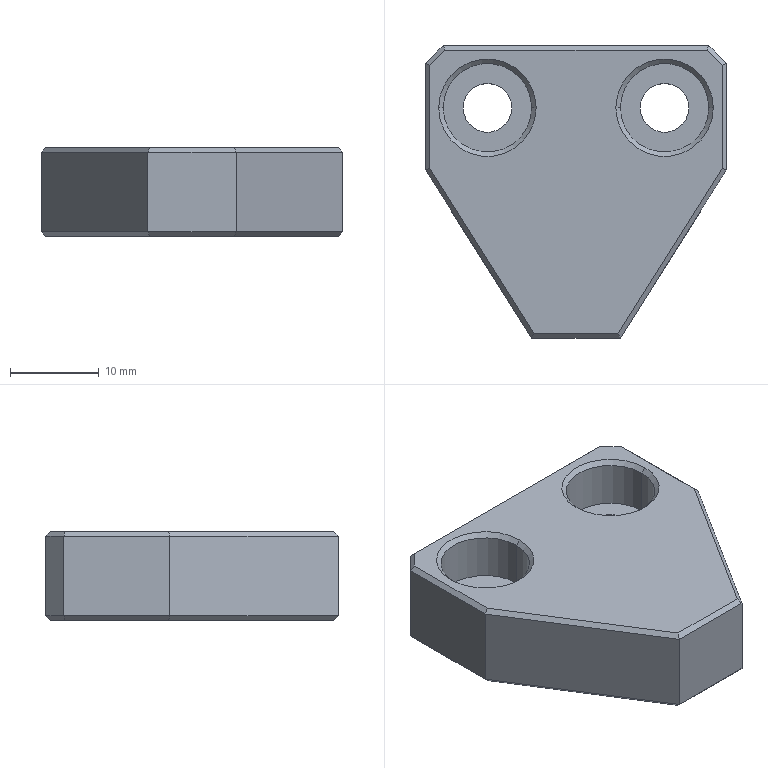Part | SolidWorks | features Chamfer 2, 3DProfileFeature 1, Extrusion 1, HoleWzd 1, ICE 1 | 1 solid | 44 faces | box 34 x 33 x 10 mm | volume 7759 mm3 | plane 28 | cone 8 | cylinder 8 | commonest cylinder face diameters 5.5 x4 10 x4
STEP:
#1=CARTESIAN_POINT('',(-15.,0.,9.5));
#2=VERTEX_POINT('',#1);
#3=CARTESIAN_POINT('',(-5.,0.,9.5));
#4=VERTEX_POINT('',#3);
#5=CARTESIAN_POINT('',(-10.,0.,9.5));
#6=DIRECTION('',(0.,0.,1.));
#7=DIRECTION('',(1.,0.,0.));
#8=AXIS2_PLACEMENT_3D('',#5,#6,#7);
#9=CIRCLE('',#8,5.);
#10=EDGE_CURVE('',#2,#4,#9,.T.);
#11=ORIENTED_EDGE('',*,*,#10,.F.);
#12=CARTESIAN_POINT('',(-15.5,0.,10.));
#13=VERTEX_POINT('',#12);
#14=CARTESIAN_POINT('',(-15.,0.,9.5));
#15=DIRECTION('',(-0.7071,0.,0.7071));
#16=VECTOR('',#15,1000.);
#17=LINE('',#14,#16);
#18=EDGE_CURVE('',#2,#13,#17,.T.);
#19=ORIENTED_EDGE('',*,*,#18,.T.);
#20=CARTESIAN_POINT('',(-4.5,0.,10.));
#21=VERTEX_POINT('',#20);
#22=CARTESIAN_POINT('',(-10.,0.,10.));
#23=DIRECTION('',(0.,0.,-1.));
#24=DIRECTION('',(1.,0.,0.));
#25=AXIS2_PLACEMENT_3D('',#22,#23,#24);
#26=CIRCLE('',#25,5.5);
#27=EDGE_CURVE('',#21,#13,#26,.T.);
#28=ORIENTED_EDGE('',*,*,#27,.F.);
#29=CARTESIAN_POINT('',(-5.,0.,9.5));
#30=DIRECTION('',(0.7071,0.,0.7071));
#31=VECTOR('',#30,1000.);
#32=LINE('',#29,#31);
#33=EDGE_CURVE('',#4,#21,#32,.T.);
#34=ORIENTED_EDGE('',*,*,#33,.F.);
#35=EDGE_LOOP('',(#11,#19,#28,#34));
#36=FACE_OUTER_BOUND('',#35,.T.);
#37=CARTESIAN_POINT('',(-10.,0.,9.5));
#38=DIRECTION('',(0.,0.,1.));
#39=DIRECTION('',(1.,0.,0.));
#40=AXIS2_PLACEMENT_3D('',#37,#38,#39);
#41=CONICAL_SURFACE('',#40,5.,0.7854);
#42=ADVANCED_FACE('',(#36),#41,.F.);
#43=CARTESIAN_POINT('',(5.,0.,9.5));
#44=VERTEX_POINT('',#43);
#45=CARTESIAN_POINT('',(15.,0.,9.5));
#46=VERTEX_POINT('',#45);
#47=CARTESIAN_POINT('',(10.,0.,9.5));
#48=DIRECTION('',(0.,0.,1.));
#49=DIRECTION('',(1.,0.,0.));
#50=AXIS2_PLACEMENT_3D('',#47,#48,#49);
#51=CIRCLE('',#50,5.);
#52=EDGE_CURVE('',#44,#46,#51,.T.);
#53=ORIENTED_EDGE('',*,*,#52,.F.);
#54=CARTESIAN_POINT('',(4.5,0.,10.));
#55=VERTEX_POINT('',#54);
#56=CARTESIAN_POINT('',(5.,0.,9.5));
#57=DIRECTION('',(-0.7071,0.,0.7071));
#58=VECTOR('',#57,1000.);
#59=LINE('',#56,#58);
#60=EDGE_CURVE('',#44,#55,#59,.T.);
#61=ORIENTED_EDGE('',*,*,#60,.T.);
#62=CARTESIAN_POINT('',(15.5,0.,10.));
#63=VERTEX_POINT('',#62);
#64=CARTESIAN_POINT('',(10.,0.,10.));
#65=DIRECTION('',(0.,0.,-1.));
#66=DIRECTION('',(1.,0.,0.));
#67=AXIS2_PLACEMENT_3D('',#64,#65,#66);
#68=CIRCLE('',#67,5.5);
#69=EDGE_CURVE('',#63,#55,#68,.T.);
#70=ORIENTED_EDGE('',*,*,#69,.F.);
#71=CARTESIAN_POINT('',(15.,0.,9.5));
#72=DIRECTION('',(0.7071,0.,0.7071));
#73=VECTOR('',#72,1000.);
#74=LINE('',#71,#73);
#75=EDGE_CURVE('',#46,#63,#74,.T.);
#76=ORIENTED_EDGE('',*,*,#75,.F.);
#77=EDGE_LOOP('',(#53,#61,#70,#76));
#78=FACE_OUTER_BOUND('',#77,.T.);
#79=CARTESIAN_POINT('',(10.,0.,9.5));
#80=DIRECTION('',(0.,0.,1.));
#81=DIRECTION('',(1.,0.,0.));
#82=AXIS2_PLACEMENT_3D('',#79,#80,#81);
#83=CONICAL_SURFACE('',#82,5.,0.7854);
#84=ADVANCED_FACE('',(#78),#83,.F.);
#85=CARTESIAN_POINT('',(-7.25,0.,0.5));
#86=VERTEX_POINT('',#85);
#87=CARTESIAN_POINT('',(-12.75,0.,0.5));
#88=VERTEX_POINT('',#87);
#89=CARTESIAN_POINT('',(-10.,0.,0.5));
#90=DIRECTION('',(0.,0.,-1.));
#91=DIRECTION('',(1.,0.,0.));
#92=AXIS2_PLACEMENT_3D('',#89,#90,#91);
#93=CIRCLE('',#92,2.75);
#94=EDGE_CURVE('',#86,#88,#93,.T.);
#95=ORIENTED_EDGE('',*,*,#94,.F.);
#96=CARTESIAN_POINT('',(-6.75,0.,0.));
#97=VERTEX_POINT('',#96);
#98=CARTESIAN_POINT('',(-6.75,0.,0.));
#99=DIRECTION('',(0.7071,0.,-0.7071));
#100=VECTOR('',#99,1000.);
#101=LINE('',#98,#100);
#102=EDGE_CURVE('',#86,#97,#101,.T.);
#103=ORIENTED_EDGE('',*,*,#102,.T.);
#104=CARTESIAN_POINT('',(-13.25,0.,0.));
#105=VERTEX_POINT('',#104);
#106=CARTESIAN_POINT('',(-10.,0.,0.));
#107=DIRECTION('',(0.,0.,1.));
#108=DIRECTION('',(1.,0.,0.));
#109=AXIS2_PLACEMENT_3D('',#106,#107,#108);
#110=CIRCLE('',#109,3.25);
#111=EDGE_CURVE('',#105,#97,#110,.T.);
#112=ORIENTED_EDGE('',*,*,#111,.F.);
#113=CARTESIAN_POINT('',(-13.25,0.,0.));
#114=DIRECTION('',(-0.7071,0.,-0.7071));
#115=VECTOR('',#114,1000.);
#116=LINE('',#113,#115);
#117=EDGE_CURVE('',#88,#105,#116,.T.);
#118=ORIENTED_EDGE('',*,*,#117,.F.);
#119=EDGE_LOOP('',(#95,#103,#112,#118));
#120=FACE_OUTER_BOUND('',#119,.T.);
#121=CARTESIAN_POINT('',(-10.,0.,0.));
#122=DIRECTION('',(0.,0.,-1.));
#123=DIRECTION('',(-1.,0.,0.));
#124=AXIS2_PLACEMENT_3D('',#121,#122,#123);
#125=CONICAL_SURFACE('',#124,3.25,0.7854);
#126=ADVANCED_FACE('',(#120),#125,.F.);
#127=CARTESIAN_POINT('',(12.75,0.,0.5));
#128=VERTEX_POINT('',#127);
#129=CARTESIAN_POINT('',(7.25,0.,0.5));
#130=VERTEX_POINT('',#129);
#131=CARTESIAN_POINT('',(10.,0.,0.5));
#132=DIRECTION('',(0.,0.,-1.));
#133=DIRECTION('',(1.,0.,0.));
#134=AXIS2_PLACEMENT_3D('',#131,#132,#133);
#135=CIRCLE('',#134,2.75);
#136=EDGE_CURVE('',#128,#130,#135,.T.);
#137=ORIENTED_EDGE('',*,*,#136,.F.);
#138=CARTESIAN_POINT('',(13.25,0.,0.));
#139=VERTEX_POINT('',#138);
#140=CARTESIAN_POINT('',(13.25,0.,0.));
#141=DIRECTION('',(0.7071,0.,-0.7071));
#142=VECTOR('',#141,1000.);
#143=LINE('',#140,#142);
#144=EDGE_CURVE('',#128,#139,#143,.T.);
#145=ORIENTED_EDGE('',*,*,#144,.T.);
#146=CARTESIAN_POINT('',(6.75,0.,0.));
#147=VERTEX_POINT('',#146);
#148=CARTESIAN_POINT('',(10.,0.,0.));
#149=DIRECTION('',(0.,0.,1.));
#150=DIRECTION('',(1.,0.,0.));
#151=AXIS2_PLACEMENT_3D('',#148,#149,#150);
#152=CIRCLE('',#151,3.25);
#153=EDGE_CURVE('',#147,#139,#152,.T.);
#154=ORIENTED_EDGE('',*,*,#153,.F.);
#155=CARTESIAN_POINT('',(6.75,0.,0.));
#156=DIRECTION('',(-0.7071,0.,-0.7071));
#157=VECTOR('',#156,1000.);
#158=LINE('',#155,#157);
#159=EDGE_CURVE('',#130,#147,#158,.T.);
#160=ORIENTED_EDGE('',*,*,#159,.F.);
#161=EDGE_LOOP('',(#137,#145,#154,#160));
#162=FACE_OUTER_BOUND('',#161,.T.);
#163=CARTESIAN_POINT('',(10.,0.,0.));
#164=DIRECTION('',(0.,0.,-1.));
#165=DIRECTION('',(-1.,0.,0.));
#166=AXIS2_PLACEMENT_3D('',#163,#164,#165);
#167=CONICAL_SURFACE('',#166,3.25,0.7854);
#168=ADVANCED_FACE('',(#162),#167,.F.);
#169=CARTESIAN_POINT('',(-15.,0.,4.3));
#170=VERTEX_POINT('',#169);
#171=CARTESIAN_POINT('',(-5.,0.,4.3));
#172=VERTEX_POINT('',#171);
#173=CARTESIAN_POINT('',(-10.,0.,4.3));
#174=DIRECTION('',(0.,0.,1.));
#175=DIRECTION('',(1.,0.,0.));
#176=AXIS2_PLACEMENT_3D('',#173,#174,#175);
#177=CIRCLE('',#176,5.);
#178=EDGE_CURVE('',#170,#172,#177,.T.);
#179=ORIENTED_EDGE('',*,*,#178,.F.);
#180=CARTESIAN_POINT('',(-15.,0.,10.));
#181=DIRECTION('',(0.,0.,1.));
#182=VECTOR('',#181,1000.);
#183=LINE('',#180,#182);
#184=EDGE_CURVE('',#170,#2,#183,.T.);
#185=ORIENTED_EDGE('',*,*,#184,.T.);
#186=ORIENTED_EDGE('',*,*,#10,.T.);
#187=CARTESIAN_POINT('',(-5.,0.,10.));
#188=DIRECTION('',(0.,0.,1.));
#189=VECTOR('',#188,1000.);
#190=LINE('',#187,#189);
#191=EDGE_CURVE('',#172,#4,#190,.T.);
#192=ORIENTED_EDGE('',*,*,#191,.F.);
#193=EDGE_LOOP('',(#179,#185,#186,#192));
#194=FACE_OUTER_BOUND('',#193,.T.);
#195=CARTESIAN_POINT('',(-10.,0.,10.));
#196=DIRECTION('',(0.,0.,1.));
#197=DIRECTION('',(1.,0.,0.));
#198=AXIS2_PLACEMENT_3D('',#195,#196,#197);
#199=CYLINDRICAL_SURFACE('',#198,5.);
#200=ADVANCED_FACE('',(#194),#199,.F.);
#201=ORIENTED_EDGE('',*,*,#94,.T.);
#202=CARTESIAN_POINT('',(-12.75,0.,4.3));
#203=VERTEX_POINT('',#202);
#204=CARTESIAN_POINT('',(-12.75,0.,10.));
#205=DIRECTION('',(0.,0.,1.));
#206=VECTOR('',#205,1000.);
#207=LINE('',#204,#206);
#208=EDGE_CURVE('',#88,#203,#207,.T.);
#209=ORIENTED_EDGE('',*,*,#208,.T.);
#210=CARTESIAN_POINT('',(-7.25,0.,4.3));
#211=VERTEX_POINT('',#210);
#212=CARTESIAN_POINT('',(-10.,0.,4.3));
#213=DIRECTION('',(0.,0.,1.));
#214=DIRECTION('',(1.,0.,0.));
#215=AXIS2_PLACEMENT_3D('',#212,#213,#214);
#216=CIRCLE('',#215,2.75);
#217=EDGE_CURVE('',#203,#211,#216,.T.);
#218=ORIENTED_EDGE('',*,*,#217,.T.);
#219=CARTESIAN_POINT('',(-7.25,0.,10.));
#220=DIRECTION('',(0.,0.,1.));
#221=VECTOR('',#220,1000.);
#222=LINE('',#219,#221);
#223=EDGE_CURVE('',#86,#211,#222,.T.);
#224=ORIENTED_EDGE('',*,*,#223,.F.);
#225=EDGE_LOOP('',(#201,#209,#218,#224));
#226=FACE_OUTER_BOUND('',#225,.T.);
#227=CARTESIAN_POINT('',(-10.,0.,10.));
#228=DIRECTION('',(0.,0.,1.));
#229=DIRECTION('',(1.,0.,0.));
#230=AXIS2_PLACEMENT_3D('',#227,#228,#229);
#231=CYLINDRICAL_SURFACE('',#230,2.75);
#232=ADVANCED_FACE('',(#226),#231,.F.);
#233=CARTESIAN_POINT('',(5.,0.,4.3));
#234=VERTEX_POINT('',#233);
#235=CARTESIAN_POINT('',(15.,0.,4.3));
#236=VERTEX_POINT('',#235);
#237=CARTESIAN_POINT('',(10.,0.,4.3));
#238=DIRECTION('',(0.,0.,1.));
#239=DIRECTION('',(1.,0.,0.));
#240=AXIS2_PLACEMENT_3D('',#237,#238,#239);
#241=CIRCLE('',#240,5.);
#242=EDGE_CURVE('',#234,#236,#241,.T.);
#243=ORIENTED_EDGE('',*,*,#242,.F.);
#244=CARTESIAN_POINT('',(5.,0.,10.));
#245=DIRECTION('',(0.,0.,1.));
#246=VECTOR('',#245,1000.);
#247=LINE('',#244,#246);
#248=EDGE_CURVE('',#234,#44,#247,.T.);
#249=ORIENTED_EDGE('',*,*,#248,.T.);
#250=ORIENTED_EDGE('',*,*,#52,.T.);
#251=CARTESIAN_POINT('',(15.,0.,10.));
#252=DIRECTION('',(0.,0.,1.));
#253=VECTOR('',#252,1000.);
#254=LINE('',#251,#253);
#255=EDGE_CURVE('',#236,#46,#254,.T.);
#256=ORIENTED_EDGE('',*,*,#255,.F.);
#257=EDGE_LOOP('',(#243,#249,#250,#256));
#258=FACE_OUTER_BOUND('',#257,.T.);
#259=CARTESIAN_POINT('',(10.,0.,10.));
#260=DIRECTION('',(0.,0.,1.));
#261=DIRECTION('',(1.,0.,0.));
#262=AXIS2_PLACEMENT_3D('',#259,#260,#261);
#263=CYLINDRICAL_SURFACE('',#262,5.);
#264=ADVANCED_FACE('',(#258),#263,.F.);
#265=ORIENTED_EDGE('',*,*,#136,.T.);
#266=CARTESIAN_POINT('',(7.25,0.,4.3));
#267=VERTEX_POINT('',#266);
#268=CARTESIAN_POINT('',(7.25,0.,10.));
#269=DIRECTION('',(0.,0.,1.));
#270=VECTOR('',#269,1000.);
#271=LINE('',#268,#270);
#272=EDGE_CURVE('',#130,#267,#271,.T.);
#273=ORIENTED_EDGE('',*,*,#272,.T.);
#274=CARTESIAN_POINT('',(12.75,0.,4.3));
#275=VERTEX_POINT('',#274);
#276=CARTESIAN_POINT('',(10.,0.,4.3));
#277=DIRECTION('',(0.,0.,1.));
#278=DIRECTION('',(1.,0.,0.));
#279=AXIS2_PLACEMENT_3D('',#276,#277,#278);
#280=CIRCLE('',#279,2.75);
#281=EDGE_CURVE('',#267,#275,#280,.T.);
#282=ORIENTED_EDGE('',*,*,#281,.T.);
#283=CARTESIAN_POINT('',(12.75,0.,10.));
#284=DIRECTION('',(0.,0.,1.));
#285=VECTOR('',#284,1000.);
#286=LINE('',#283,#285);
#287=EDGE_CURVE('',#128,#275,#286,.T.);
#288=ORIENTED_EDGE('',*,*,#287,.F.);
#289=EDGE_LOOP('',(#265,#273,#282,#288));
#290=FACE_OUTER_BOUND('',#289,.T.);
#291=CARTESIAN_POINT('',(10.,0.,10.));
#292=DIRECTION('',(0.,0.,1.));
#293=DIRECTION('',(1.,0.,0.));
#294=AXIS2_PLACEMENT_3D('',#291,#292,#293);
#295=CYLINDRICAL_SURFACE('',#294,2.75);
#296=ADVANCED_FACE('',(#290),#295,.F.);
#297=CARTESIAN_POINT('',(-17.,5.,9.5));
#298=VERTEX_POINT('',#297);
#299=CARTESIAN_POINT('',(-17.,5.,0.5));
#300=VERTEX_POINT('',#299);
#301=CARTESIAN_POINT('',(-17.,5.,10.));
#302=DIRECTION('',(0.,0.,-1.));
#303=VECTOR('',#302,1000.);
#304=LINE('',#301,#303);
#305=EDGE_CURVE('',#298,#300,#304,.T.);
#306=ORIENTED_EDGE('',*,*,#305,.T.);
#307=CARTESIAN_POINT('',(-17.,-7.,0.5));
#308=VERTEX_POINT('',#307);
#309=CARTESIAN_POINT('',(-17.,-7.,0.5));
#310=DIRECTION('',(0.,-1.,0.));
#311=VECTOR('',#310,1000.);
#312=LINE('',#309,#311);
#313=EDGE_CURVE('',#300,#308,#312,.T.);
#314=ORIENTED_EDGE('',*,*,#313,.T.);
#315=CARTESIAN_POINT('',(-17.,-7.,9.5));
#316=VERTEX_POINT('',#315);
#317=CARTESIAN_POINT('',(-17.,-7.,10.));
#318=DIRECTION('',(0.,0.,-1.));
#319=VECTOR('',#318,1000.);
#320=LINE('',#317,#319);
#321=EDGE_CURVE('',#316,#308,#320,.T.);
#322=ORIENTED_EDGE('',*,*,#321,.F.);
#323=CARTESIAN_POINT('',(-17.,5.,9.5));
#324=DIRECTION('',(0.,1.,0.));
#325=VECTOR('',#324,1000.);
#326=LINE('',#323,#325);
#327=EDGE_CURVE('',#316,#298,#326,.T.);
#328=ORIENTED_EDGE('',*,*,#327,.T.);
#329=EDGE_LOOP('',(#306,#314,#322,#328));
#330=FACE_OUTER_BOUND('',#329,.T.);
#331=CARTESIAN_POINT('',(-17.,-7.,10.));
#332=DIRECTION('',(1.,0.,0.));
#333=DIRECTION('',(0.,0.,-1.));
#334=AXIS2_PLACEMENT_3D('',#331,#332,#333);
#335=PLANE('',#334);
#336=ADVANCED_FACE('',(#330),#335,.F.);
#337=CARTESIAN_POINT('',(17.,-7.,9.5));
#338=VERTEX_POINT('',#337);
#339=CARTESIAN_POINT('',(17.,-7.,0.5));
#340=VERTEX_POINT('',#339);
#341=CARTESIAN_POINT('',(17.,-7.,10.));
#342=DIRECTION('',(0.,0.,-1.));
#343=VECTOR('',#342,1000.);
#344=LINE('',#341,#343);
#345=EDGE_CURVE('',#338,#340,#344,.T.);
#346=ORIENTED_EDGE('',*,*,#345,.T.);
#347=CARTESIAN_POINT('',(17.,5.,0.5));
#348=VERTEX_POINT('',#347);
#349=CARTESIAN_POINT('',(17.,-7.,0.5));
#350=DIRECTION('',(0.,1.,0.));
#351=VECTOR('',#350,1000.);
#352=LINE('',#349,#351);
#353=EDGE_CURVE('',#340,#348,#352,.T.);
#354=ORIENTED_EDGE('',*,*,#353,.T.);
#355=CARTESIAN_POINT('',(17.,5.,9.5));
#356=VERTEX_POINT('',#355);
#357=CARTESIAN_POINT('',(17.,5.,10.));
#358=DIRECTION('',(0.,0.,1.));
#359=VECTOR('',#358,1000.);
#360=LINE('',#357,#359);
#361=EDGE_CURVE('',#348,#356,#360,.T.);
#362=ORIENTED_EDGE('',*,*,#361,.T.);
#363=CARTESIAN_POINT('',(17.,-7.,9.5));
#364=DIRECTION('',(0.,-1.,0.));
#365=VECTOR('',#364,1000.);
#366=LINE('',#363,#365);
#367=EDGE_CURVE('',#356,#338,#366,.T.);
#368=ORIENTED_EDGE('',*,*,#367,.T.);
#369=EDGE_LOOP('',(#346,#354,#362,#368));
#370=FACE_OUTER_BOUND('',#369,.T.);
#371=CARTESIAN_POINT('',(17.,-7.,10.));
#372=DIRECTION('',(-1.,0.,0.));
#373=DIRECTION('',(0.,0.,1.));
#374=AXIS2_PLACEMENT_3D('',#371,#372,#373);
#375=PLANE('',#374);
#376=ADVANCED_FACE('',(#370),#375,.F.);
#377=CARTESIAN_POINT('',(15.,7.,9.5));
#378=VERTEX_POINT('',#377);
#379=CARTESIAN_POINT('',(15.,7.,0.5));
#380=VERTEX_POINT('',#379);
#381=CARTESIAN_POINT('',(15.,7.,10.));
#382=DIRECTION('',(0.,0.,-1.));
#383=VECTOR('',#382,1000.);
#384=LINE('',#381,#383);
#385=EDGE_CURVE('',#378,#380,#384,.T.);
#386=ORIENTED_EDGE('',*,*,#385,.T.);
#387=CARTESIAN_POINT('',(-15.,7.,0.5));
#388=VERTEX_POINT('',#387);
#389=CARTESIAN_POINT('',(17.,7.,0.5));
#390=DIRECTION('',(-1.,0.,0.));
#391=VECTOR('',#390,1000.);
#392=LINE('',#389,#391);
#393=EDGE_CURVE('',#380,#388,#392,.T.);
#394=ORIENTED_EDGE('',*,*,#393,.T.);
#395=CARTESIAN_POINT('',(-15.,7.,9.5));
#396=VERTEX_POINT('',#395);
#397=CARTESIAN_POINT('',(-15.,7.,10.));
#398=DIRECTION('',(0.,0.,1.));
#399=VECTOR('',#398,1000.);
#400=LINE('',#397,#399);
#401=EDGE_CURVE('',#388,#396,#400,.T.);
#402=ORIENTED_EDGE('',*,*,#401,.T.);
#403=CARTESIAN_POINT('',(15.,7.,9.5));
#404=DIRECTION('',(1.,0.,0.));
#405=VECTOR('',#404,1000.);
#406=LINE('',#403,#405);
#407=EDGE_CURVE('',#396,#378,#406,.T.);
#408=ORIENTED_EDGE('',*,*,#407,.T.);
#409=EDGE_LOOP('',(#386,#394,#402,#408));
#410=FACE_OUTER_BOUND('',#409,.T.);
#411=CARTESIAN_POINT('',(17.,7.,10.));
#412=DIRECTION('',(0.,-1.,0.));
#413=DIRECTION('',(1.,0.,0.));
#414=AXIS2_PLACEMENT_3D('',#411,#412,#413);
#415=PLANE('',#414);
#416=ADVANCED_FACE('',(#410),#415,.F.);
#417=CARTESIAN_POINT('',(16.5,-6.855,10.));
#418=VERTEX_POINT('',#417);
#419=CARTESIAN_POINT('',(16.5,4.793,10.));
#420=VERTEX_POINT('',#419);
#421=CARTESIAN_POINT('',(16.5,5.,10.));
#422=DIRECTION('',(0.,1.,0.));
#423=VECTOR('',#422,1000.);
#424=LINE('',#421,#423);
#425=EDGE_CURVE('',#418,#420,#424,.T.);
#426=ORIENTED_EDGE('',*,*,#425,.T.);
#427=CARTESIAN_POINT('',(14.793,6.5,10.));
#428=VERTEX_POINT('',#427);
#429=CARTESIAN_POINT('',(10.646,10.646,10.));
#430=DIRECTION('',(-0.7071,0.7071,0.));
#431=VECTOR('',#430,1000.);
#432=LINE('',#429,#431);
#433=EDGE_CURVE('',#420,#428,#432,.T.);
#434=ORIENTED_EDGE('',*,*,#433,.T.);
#435=CARTESIAN_POINT('',(-14.793,6.5,10.));
#436=VERTEX_POINT('',#435);
#437=CARTESIAN_POINT('',(-15.,6.5,10.));
#438=DIRECTION('',(-1.,0.,0.));
#439=VECTOR('',#438,1000.);
#440=LINE('',#437,#439);
#441=EDGE_CURVE('',#428,#436,#440,.T.);
#442=ORIENTED_EDGE('',*,*,#441,.T.);
#443=CARTESIAN_POINT('',(-16.5,4.793,10.));
#444=VERTEX_POINT('',#443);
#445=CARTESIAN_POINT('',(-10.646,10.646,10.));
#446=DIRECTION('',(-0.7071,-0.7071,0.));
#447=VECTOR('',#446,1000.);
#448=LINE('',#445,#447);
#449=EDGE_CURVE('',#436,#444,#448,.T.);
#450=ORIENTED_EDGE('',*,*,#449,.T.);
#451=CARTESIAN_POINT('',(-16.5,-6.855,10.));
#452=VERTEX_POINT('',#451);
#453=CARTESIAN_POINT('',(-16.5,-7.,10.));
#454=DIRECTION('',(0.,-1.,0.));
#455=VECTOR('',#454,1000.);
#456=LINE('',#453,#455);
#457=EDGE_CURVE('',#444,#452,#456,.T.);
#458=ORIENTED_EDGE('',*,*,#457,.T.);
#459=CARTESIAN_POINT('',(-4.724,-25.5,10.));
#460=VERTEX_POINT('',#459);
#461=CARTESIAN_POINT('',(-14.89,-9.404,10.));
#462=DIRECTION('',(0.534,-0.8455,0.));
#463=VECTOR('',#462,1000.);
#464=LINE('',#461,#463);
#465=EDGE_CURVE('',#452,#460,#464,.T.);
#466=ORIENTED_EDGE('',*,*,#465,.T.);
#467=CARTESIAN_POINT('',(4.724,-25.5,10.));
#468=VERTEX_POINT('',#467);
#469=CARTESIAN_POINT('',(0.,-25.5,10.));
#470=DIRECTION('',(1.,0.,0.));
#471=VECTOR('',#470,1000.);
#472=LINE('',#469,#471);
#473=EDGE_CURVE('',#460,#468,#472,.T.);
#474=ORIENTED_EDGE('',*,*,#473,.T.);
#475=CARTESIAN_POINT('',(14.89,-9.404,10.));
#476=DIRECTION('',(0.534,0.8455,0.));
#477=VECTOR('',#476,1000.);
#478=LINE('',#475,#477);
#479=EDGE_CURVE('',#468,#418,#478,.T.);
#480=ORIENTED_EDGE('',*,*,#479,.T.);
#481=EDGE_LOOP('',(#426,#434,#442,#450,#458,#466,#474,#480));
#482=FACE_OUTER_BOUND('',#481,.T.);
#483=ORIENTED_EDGE('',*,*,#69,.T.);
#484=CARTESIAN_POINT('',(10.,0.,10.));
#485=DIRECTION('',(0.,0.,-1.));
#486=DIRECTION('',(1.,0.,0.));
#487=AXIS2_PLACEMENT_3D('',#484,#485,#486);
#488=CIRCLE('',#487,5.5);
#489=EDGE_CURVE('',#55,#63,#488,.T.);
#490=ORIENTED_EDGE('',*,*,#489,.T.);
#491=EDGE_LOOP('',(#483,#490));
#492=FACE_BOUND('',#491,.T.);
#493=ORIENTED_EDGE('',*,*,#27,.T.);
#494=CARTESIAN_POINT('',(-10.,0.,10.));
#495=DIRECTION('',(0.,0.,-1.));
#496=DIRECTION('',(1.,0.,0.));
#497=AXIS2_PLACEMENT_3D('',#494,#495,#496);
#498=CIRCLE('',#497,5.5);
#499=EDGE_CURVE('',#13,#21,#498,.T.);
#500=ORIENTED_EDGE('',*,*,#499,.T.);
#501=EDGE_LOOP('',(#493,#500));
#502=FACE_BOUND('',#501,.T.);
#503=CARTESIAN_POINT('',(0.,0.,10.));
#504=DIRECTION('',(0.,0.,1.));
#505=DIRECTION('',(1.,0.,0.));
#506=AXIS2_PLACEMENT_3D('',#503,#504,#505);
#507=PLANE('',#506);
#508=ADVANCED_FACE('',(#482,#492,#502),#507,.T.);
#509=CARTESIAN_POINT('',(4.724,-25.5,0.));
#510=VERTEX_POINT('',#509);
#511=CARTESIAN_POINT('',(-4.724,-25.5,0.));
#512=VERTEX_POINT('',#511);
#513=CARTESIAN_POINT('',(-5.,-25.5,0.));
#514=DIRECTION('',(-1.,0.,0.));
#515=VECTOR('',#514,1000.);
#516=LINE('',#513,#515);
#517=EDGE_CURVE('',#510,#512,#516,.T.);
#518=ORIENTED_EDGE('',*,*,#517,.T.);
#519=CARTESIAN_POINT('',(-16.5,-6.855,0.));
#520=VERTEX_POINT('',#519);
#521=CARTESIAN_POINT('',(-16.577,-6.733,0.));
#522=DIRECTION('',(-0.534,0.8455,0.));
#523=VECTOR('',#522,1000.);
#524=LINE('',#521,#523);
#525=EDGE_CURVE('',#512,#520,#524,.T.);
#526=ORIENTED_EDGE('',*,*,#525,.T.);
#527=CARTESIAN_POINT('',(-16.5,4.793,0.));
#528=VERTEX_POINT('',#527);
#529=CARTESIAN_POINT('',(-16.5,0.,0.));
#530=DIRECTION('',(0.,1.,0.));
#531=VECTOR('',#530,1000.);
#532=LINE('',#529,#531);
#533=EDGE_CURVE('',#520,#528,#532,.T.);
#534=ORIENTED_EDGE('',*,*,#533,.T.);
#535=CARTESIAN_POINT('',(-14.793,6.5,0.));
#536=VERTEX_POINT('',#535);
#537=CARTESIAN_POINT('',(-14.646,6.646,0.));
#538=DIRECTION('',(0.7071,0.7071,0.));
#539=VECTOR('',#538,1000.);
#540=LINE('',#537,#539);
#541=EDGE_CURVE('',#528,#536,#540,.T.);
#542=ORIENTED_EDGE('',*,*,#541,.T.);
#543=CARTESIAN_POINT('',(14.793,6.5,0.));
#544=VERTEX_POINT('',#543);
#545=CARTESIAN_POINT('',(0.,6.5,0.));
#546=DIRECTION('',(1.,0.,0.));
#547=VECTOR('',#546,1000.);
#548=LINE('',#545,#547);
#549=EDGE_CURVE('',#536,#544,#548,.T.);
#550=ORIENTED_EDGE('',*,*,#549,.T.);
#551=CARTESIAN_POINT('',(16.5,4.793,0.));
#552=VERTEX_POINT('',#551);
#553=CARTESIAN_POINT('',(16.646,4.646,0.));
#554=DIRECTION('',(0.7071,-0.7071,0.));
#555=VECTOR('',#554,1000.);
#556=LINE('',#553,#555);
#557=EDGE_CURVE('',#544,#552,#556,.T.);
#558=ORIENTED_EDGE('',*,*,#557,.T.);
#559=CARTESIAN_POINT('',(16.5,-6.855,0.));
#560=VERTEX_POINT('',#559);
#561=CARTESIAN_POINT('',(16.5,0.,0.));
#562=DIRECTION('',(0.,-1.,0.));
#563=VECTOR('',#562,1000.);
#564=LINE('',#561,#563);
#565=EDGE_CURVE('',#552,#560,#564,.T.);
#566=ORIENTED_EDGE('',*,*,#565,.T.);
#567=CARTESIAN_POINT('',(4.577,-25.733,0.));
#568=DIRECTION('',(-0.534,-0.8455,0.));
#569=VECTOR('',#568,1000.);
#570=LINE('',#567,#569);
#571=EDGE_CURVE('',#560,#510,#570,.T.);
#572=ORIENTED_EDGE('',*,*,#571,.T.);
#573=EDGE_LOOP('',(#518,#526,#534,#542,#550,#558,#566,#572));
#574=FACE_OUTER_BOUND('',#573,.T.);
#575=ORIENTED_EDGE('',*,*,#153,.T.);
#576=CARTESIAN_POINT('',(10.,0.,0.));
#577=DIRECTION('',(0.,0.,1.));
#578=DIRECTION('',(1.,0.,0.));
#579=AXIS2_PLACEMENT_3D('',#576,#577,#578);
#580=CIRCLE('',#579,3.25);
#581=EDGE_CURVE('',#139,#147,#580,.T.);
#582=ORIENTED_EDGE('',*,*,#581,.T.);
#583=EDGE_LOOP('',(#575,#582));
#584=FACE_BOUND('',#583,.T.);
#585=ORIENTED_EDGE('',*,*,#111,.T.);
#586=CARTESIAN_POINT('',(-10.,0.,0.));
#587=DIRECTION('',(0.,0.,1.));
#588=DIRECTION('',(1.,0.,0.));
#589=AXIS2_PLACEMENT_3D('',#586,#587,#588);
#590=CIRCLE('',#589,3.25);
#591=EDGE_CURVE('',#97,#105,#590,.T.);
#592=ORIENTED_EDGE('',*,*,#591,.T.);
#593=EDGE_LOOP('',(#585,#592));
#594=FACE_BOUND('',#593,.T.);
#595=CARTESIAN_POINT('',(0.,0.,0.));
#596=DIRECTION('',(0.,0.,1.));
#597=DIRECTION('',(1.,0.,0.));
#598=AXIS2_PLACEMENT_3D('',#595,#596,#597);
#599=PLANE('',#598);
#600=ADVANCED_FACE('',(#574,#584,#594),#599,.F.);
#601=ORIENTED_EDGE('',*,*,#272,.F.);
#602=CARTESIAN_POINT('',(10.,0.,0.5));
#603=DIRECTION('',(0.,0.,-1.));
#604=DIRECTION('',(1.,0.,0.));
#605=AXIS2_PLACEMENT_3D('',#602,#603,#604);
#606=CIRCLE('',#605,2.75);
#607=EDGE_CURVE('',#130,#128,#606,.T.);
#608=ORIENTED_EDGE('',*,*,#607,.T.);
#609=ORIENTED_EDGE('',*,*,#287,.T.);
#610=CARTESIAN_POINT('',(10.,0.,4.3));
#611=DIRECTION('',(0.,0.,1.));
#612=DIRECTION('',(1.,0.,0.));
#613=AXIS2_PLACEMENT_3D('',#610,#611,#612);
#614=CIRCLE('',#613,2.75);
#615=EDGE_CURVE('',#275,#267,#614,.T.);
#616=ORIENTED_EDGE('',*,*,#615,.T.);
#617=EDGE_LOOP('',(#601,#608,#609,#616));
#618=FACE_OUTER_BOUND('',#617,.T.);
#619=CARTESIAN_POINT('',(10.,0.,10.));
#620=DIRECTION('',(0.,0.,1.));
#621=DIRECTION('',(1.,0.,0.));
#622=AXIS2_PLACEMENT_3D('',#619,#620,#621);
#623=CYLINDRICAL_SURFACE('',#622,2.75);
#624=ADVANCED_FACE('',(#618),#623,.F.);
#625=ORIENTED_EDGE('',*,*,#615,.F.);
#626=ORIENTED_EDGE('',*,*,#281,.F.);
#627=EDGE_LOOP('',(#625,#626));
#628=FACE_BOUND('',#627,.T.);
#629=CARTESIAN_POINT('',(10.,0.,4.3));
#630=DIRECTION('',(0.,0.,1.));
#631=DIRECTION('',(1.,0.,0.));
#632=AXIS2_PLACEMENT_3D('',#629,#630,#631);
#633=CIRCLE('',#632,5.);
#634=EDGE_CURVE('',#236,#234,#633,.T.);
#635=ORIENTED_EDGE('',*,*,#634,.T.);
#636=ORIENTED_EDGE('',*,*,#242,.T.);
#637=EDGE_LOOP('',(#635,#636));
#638=FACE_OUTER_BOUND('',#637,.T.);
#639=CARTESIAN_POINT('',(12.75,0.,4.3));
#640=DIRECTION('',(0.,0.,-1.));
#641=DIRECTION('',(-1.,0.,0.));
#642=AXIS2_PLACEMENT_3D('',#639,#640,#641);
#643=PLANE('',#642);
#644=ADVANCED_FACE('',(#628,#638),#643,.F.);
#645=ORIENTED_EDGE('',*,*,#248,.F.);
#646=ORIENTED_EDGE('',*,*,#634,.F.);
#647=ORIENTED_EDGE('',*,*,#255,.T.);
#648=CARTESIAN_POINT('',(10.,0.,9.5));
#649=DIRECTION('',(0.,0.,1.));
#650=DIRECTION('',(1.,0.,0.));
#651=AXIS2_PLACEMENT_3D('',#648,#649,#650);
#652=CIRCLE('',#651,5.);
#653=EDGE_CURVE('',#46,#44,#652,.T.);
#654=ORIENTED_EDGE('',*,*,#653,.T.);
#655=EDGE_LOOP('',(#645,#646,#647,#654));
#656=FACE_OUTER_BOUND('',#655,.T.);
#657=CARTESIAN_POINT('',(10.,0.,10.));
#658=DIRECTION('',(0.,0.,1.));
#659=DIRECTION('',(1.,0.,0.));
#660=AXIS2_PLACEMENT_3D('',#657,#658,#659);
#661=CYLINDRICAL_SURFACE('',#660,5.);
#662=ADVANCED_FACE('',(#656),#661,.F.);
#663=ORIENTED_EDGE('',*,*,#208,.F.);
#664=CARTESIAN_POINT('',(-10.,0.,0.5));
#665=DIRECTION('',(0.,0.,-1.));
#666=DIRECTION('',(1.,0.,0.));
#667=AXIS2_PLACEMENT_3D('',#664,#665,#666);
#668=CIRCLE('',#667,2.75);
#669=EDGE_CURVE('',#88,#86,#668,.T.);
#670=ORIENTED_EDGE('',*,*,#669,.T.);
#671=ORIENTED_EDGE('',*,*,#223,.T.);
#672=CARTESIAN_POINT('',(-10.,0.,4.3));
#673=DIRECTION('',(0.,0.,1.));
#674=DIRECTION('',(1.,0.,0.));
#675=AXIS2_PLACEMENT_3D('',#672,#673,#674);
#676=CIRCLE('',#675,2.75);
#677=EDGE_CURVE('',#211,#203,#676,.T.);
#678=ORIENTED_EDGE('',*,*,#677,.T.);
#679=EDGE_LOOP('',(#663,#670,#671,#678));
#680=FACE_OUTER_BOUND('',#679,.T.);
#681=CARTESIAN_POINT('',(-10.,0.,10.));
#682=DIRECTION('',(0.,0.,1.));
#683=DIRECTION('',(1.,0.,0.));
#684=AXIS2_PLACEMENT_3D('',#681,#682,#683);
#685=CYLINDRICAL_SURFACE('',#684,2.75);
#686=ADVANCED_FACE('',(#680),#685,.F.);
#687=ORIENTED_EDGE('',*,*,#677,.F.);
#688=ORIENTED_EDGE('',*,*,#217,.F.);
#689=EDGE_LOOP('',(#687,#688));
#690=FACE_BOUND('',#689,.T.);
#691=CARTESIAN_POINT('',(-10.,0.,4.3));
#692=DIRECTION('',(0.,0.,1.));
#693=DIRECTION('',(1.,0.,0.));
#694=AXIS2_PLACEMENT_3D('',#691,#692,#693);
#695=CIRCLE('',#694,5.);
#696=EDGE_CURVE('',#172,#170,#695,.T.);
#697=ORIENTED_EDGE('',*,*,#696,.T.);
#698=ORIENTED_EDGE('',*,*,#178,.T.);
#699=EDGE_LOOP('',(#697,#698));
#700=FACE_OUTER_BOUND('',#699,.T.);
#701=CARTESIAN_POINT('',(-7.25,0.,4.3));
#702=DIRECTION('',(0.,0.,-1.));
#703=DIRECTION('',(-1.,0.,0.));
#704=AXIS2_PLACEMENT_3D('',#701,#702,#703);
#705=PLANE('',#704);
#706=ADVANCED_FACE('',(#690,#700),#705,.F.);
#707=ORIENTED_EDGE('',*,*,#184,.F.);
#708=ORIENTED_EDGE('',*,*,#696,.F.);
#709=ORIENTED_EDGE('',*,*,#191,.T.);
#710=CARTESIAN_POINT('',(-10.,0.,9.5));
#711=DIRECTION('',(0.,0.,1.));
#712=DIRECTION('',(1.,0.,0.));
#713=AXIS2_PLACEMENT_3D('',#710,#711,#712);
#714=CIRCLE('',#713,5.);
#715=EDGE_CURVE('',#4,#2,#714,.T.);
#716=ORIENTED_EDGE('',*,*,#715,.T.);
#717=EDGE_LOOP('',(#707,#708,#709,#716));
#718=FACE_OUTER_BOUND('',#717,.T.);
#719=CARTESIAN_POINT('',(-10.,0.,10.));
#720=DIRECTION('',(0.,0.,1.));
#721=DIRECTION('',(1.,0.,0.));
#722=AXIS2_PLACEMENT_3D('',#719,#720,#721);
#723=CYLINDRICAL_SURFACE('',#722,5.);
#724=ADVANCED_FACE('',(#718),#723,.F.);
#725=CARTESIAN_POINT('',(5.,-26.,0.5));
#726=VERTEX_POINT('',#725);
#727=CARTESIAN_POINT('',(5.,-26.,9.5));
#728=VERTEX_POINT('',#727);
#729=CARTESIAN_POINT('',(5.,-26.,-38.949));
#730=DIRECTION('',(0.,0.,1.));
#731=VECTOR('',#730,1000.);
#732=LINE('',#729,#731);
#733=EDGE_CURVE('',#726,#728,#732,.T.);
#734=ORIENTED_EDGE('',*,*,#733,.F.);
#735=CARTESIAN_POINT('',(17.,-7.,0.5));
#736=DIRECTION('',(0.534,0.8455,0.));
#737=VECTOR('',#736,1000.);
#738=LINE('',#735,#737);
#739=EDGE_CURVE('',#726,#340,#738,.T.);
#740=ORIENTED_EDGE('',*,*,#739,.T.);
#741=ORIENTED_EDGE('',*,*,#345,.F.);
#742=CARTESIAN_POINT('',(5.,-26.,9.5));
#743=DIRECTION('',(-0.534,-0.8455,0.));
#744=VECTOR('',#743,1000.);
#745=LINE('',#742,#744);
#746=EDGE_CURVE('',#338,#728,#745,.T.);
#747=ORIENTED_EDGE('',*,*,#746,.T.);
#748=EDGE_LOOP('',(#734,#740,#741,#747));
#749=FACE_OUTER_BOUND('',#748,.T.);
#750=CARTESIAN_POINT('',(5.,-26.,-38.949));
#751=DIRECTION('',(0.8455,-0.534,0.));
#752=DIRECTION('',(0.534,0.8455,0.));
#753=AXIS2_PLACEMENT_3D('',#750,#751,#752);
#754=PLANE('',#753);
#755=ADVANCED_FACE('',(#749),#754,.T.);
#756=CARTESIAN_POINT('',(-5.,-26.,0.5));
#757=VERTEX_POINT('',#756);
#758=CARTESIAN_POINT('',(-5.,-26.,9.5));
#759=VERTEX_POINT('',#758);
#760=CARTESIAN_POINT('',(-5.,-26.,-38.949));
#761=DIRECTION('',(0.,0.,1.));
#762=VECTOR('',#761,1000.);
#763=LINE('',#760,#762);
#764=EDGE_CURVE('',#757,#759,#763,.T.);
#765=ORIENTED_EDGE('',*,*,#764,.F.);
#766=CARTESIAN_POINT('',(5.,-26.,0.5));
#767=DIRECTION('',(1.,0.,0.));
#768=VECTOR('',#767,1000.);
#769=LINE('',#766,#768);
#770=EDGE_CURVE('',#757,#726,#769,.T.);
#771=ORIENTED_EDGE('',*,*,#770,.T.);
#772=ORIENTED_EDGE('',*,*,#733,.T.);
#773=CARTESIAN_POINT('',(-5.,-26.,9.5));
#774=DIRECTION('',(-1.,0.,0.));
#775=VECTOR('',#774,1000.);
#776=LINE('',#773,#775);
#777=EDGE_CURVE('',#728,#759,#776,.T.);
#778=ORIENTED_EDGE('',*,*,#777,.T.);
#779=EDGE_LOOP('',(#765,#771,#772,#778));
#780=FACE_OUTER_BOUND('',#779,.T.);
#781=CARTESIAN_POINT('',(-5.,-26.,-38.949));
#782=DIRECTION('',(0.,-1.,0.));
#783=DIRECTION('',(0.,0.,-1.));
#784=AXIS2_PLACEMENT_3D('',#781,#782,#783);
#785=PLANE('',#784);
#786=ADVANCED_FACE('',(#780),#785,.T.);
#787=ORIENTED_EDGE('',*,*,#321,.T.);
#788=CARTESIAN_POINT('',(-5.,-26.,0.5));
#789=DIRECTION('',(0.534,-0.8455,0.));
#790=VECTOR('',#789,1000.);
#791=LINE('',#788,#790);
#792=EDGE_CURVE('',#308,#757,#791,.T.);
#793=ORIENTED_EDGE('',*,*,#792,.T.);
#794=ORIENTED_EDGE('',*,*,#764,.T.);
#795=CARTESIAN_POINT('',(-17.,-7.,9.5));
#796=DIRECTION('',(-0.534,0.8455,0.));
#797=VECTOR('',#796,1000.);
#798=LINE('',#795,#797);
#799=EDGE_CURVE('',#759,#316,#798,.T.);
#800=ORIENTED_EDGE('',*,*,#799,.T.);
#801=EDGE_LOOP('',(#787,#793,#794,#800));
#802=FACE_OUTER_BOUND('',#801,.T.);
#803=CARTESIAN_POINT('',(-17.,-7.,-38.949));
#804=DIRECTION('',(-0.8455,-0.534,0.));
#805=DIRECTION('',(0.534,-0.8455,0.));
#806=AXIS2_PLACEMENT_3D('',#803,#804,#805);
#807=PLANE('',#806);
#808=ADVANCED_FACE('',(#802),#807,.T.);
#809=ORIENTED_EDGE('',*,*,#401,.F.);
#810=CARTESIAN_POINT('',(-17.,5.,0.5));
#811=DIRECTION('',(-0.7071,-0.7071,0.));
#812=VECTOR('',#811,1000.);
#813=LINE('',#810,#812);
#814=EDGE_CURVE('',#388,#300,#813,.T.);
#815=ORIENTED_EDGE('',*,*,#814,.T.);
#816=ORIENTED_EDGE('',*,*,#305,.F.);
#817=CARTESIAN_POINT('',(-17.,5.,9.5));
#818=DIRECTION('',(0.7071,0.7071,0.));
#819=VECTOR('',#818,1000.);
#820=LINE('',#817,#819);
#821=EDGE_CURVE('',#298,#396,#820,.T.);
#822=ORIENTED_EDGE('',*,*,#821,.T.);
#823=EDGE_LOOP('',(#809,#815,#816,#822));
#824=FACE_OUTER_BOUND('',#823,.T.);
#825=CARTESIAN_POINT('',(-17.,5.,10.));
#826=DIRECTION('',(0.7071,-0.7071,0.));
#827=DIRECTION('',(0.,0.,-1.));
#828=AXIS2_PLACEMENT_3D('',#825,#826,#827);
#829=PLANE('',#828);
#830=ADVANCED_FACE('',(#824),#829,.F.);
#831=ORIENTED_EDGE('',*,*,#361,.F.);
#832=CARTESIAN_POINT('',(15.,7.,0.5));
#833=DIRECTION('',(-0.7071,0.7071,0.));
#834=VECTOR('',#833,1000.);
#835=LINE('',#832,#834);
#836=EDGE_CURVE('',#348,#380,#835,.T.);
#837=ORIENTED_EDGE('',*,*,#836,.T.);
#838=ORIENTED_EDGE('',*,*,#385,.F.);
#839=CARTESIAN_POINT('',(15.,7.,9.5));
#840=DIRECTION('',(0.7071,-0.7071,0.));
#841=VECTOR('',#840,1000.);
#842=LINE('',#839,#841);
#843=EDGE_CURVE('',#378,#356,#842,.T.);
#844=ORIENTED_EDGE('',*,*,#843,.T.);
#845=EDGE_LOOP('',(#831,#837,#838,#844));
#846=FACE_OUTER_BOUND('',#845,.T.);
#847=CARTESIAN_POINT('',(15.,7.,10.));
#848=DIRECTION('',(-0.7071,-0.7071,0.));
#849=DIRECTION('',(0.,0.,-1.));
#850=AXIS2_PLACEMENT_3D('',#847,#848,#849);
#851=PLANE('',#850);
#852=ADVANCED_FACE('',(#846),#851,.F.);
#853=CARTESIAN_POINT('',(15.158,7.381,0.8815));
#854=DIRECTION('',(-0.2811,-0.6786,-0.6786));
#855=VECTOR('',#854,1000.);
#856=LINE('',#853,#855);
#857=EDGE_CURVE('',#380,#544,#856,.T.);
#858=ORIENTED_EDGE('',*,*,#857,.F.);
#859=ORIENTED_EDGE('',*,*,#836,.F.);
#860=CARTESIAN_POINT('',(14.921,4.139,-1.579));
#861=DIRECTION('',(0.6786,0.2811,0.6786));
#862=VECTOR('',#861,1000.);
#863=LINE('',#860,#862);
#864=EDGE_CURVE('',#552,#348,#863,.T.);
#865=ORIENTED_EDGE('',*,*,#864,.F.);
#866=ORIENTED_EDGE('',*,*,#557,.F.);
#867=EDGE_LOOP('',(#858,#859,#865,#866));
#868=FACE_OUTER_BOUND('',#867,.T.);
#869=CARTESIAN_POINT('',(10.646,10.646,0.));
#870=DIRECTION('',(-0.5,-0.5,0.7071));
#871=DIRECTION('',(0.7071,-0.7071,0.));
#872=AXIS2_PLACEMENT_3D('',#869,#870,#871);
#873=PLANE('',#872);
#874=ADVANCED_FACE('',(#868),#873,.F.);
#875=ORIENTED_EDGE('',*,*,#864,.T.);
#876=ORIENTED_EDGE('',*,*,#353,.F.);
#877=CARTESIAN_POINT('',(17.,-7.,0.5));
#878=DIRECTION('',(0.6928,-0.2004,0.6928));
#879=VECTOR('',#878,1000.);
#880=LINE('',#877,#879);
#881=EDGE_CURVE('',#560,#340,#880,.T.);
#882=ORIENTED_EDGE('',*,*,#881,.F.);
#883=ORIENTED_EDGE('',*,*,#565,.F.);
#884=EDGE_LOOP('',(#875,#876,#882,#883));
#885=FACE_OUTER_BOUND('',#884,.T.);
#886=CARTESIAN_POINT('',(17.,-7.,0.5));
#887=DIRECTION('',(-0.7071,0.,0.7071));
#888=DIRECTION('',(0.,1.,0.));
#889=AXIS2_PLACEMENT_3D('',#886,#887,#888);
#890=PLANE('',#889);
#891=ADVANCED_FACE('',(#885),#890,.F.);
#892=ORIENTED_EDGE('',*,*,#857,.T.);
#893=ORIENTED_EDGE('',*,*,#549,.F.);
#894=CARTESIAN_POINT('',(-15.256,7.619,1.119));
#895=DIRECTION('',(0.2811,-0.6786,-0.6786));
#896=VECTOR('',#895,1000.);
#897=LINE('',#894,#896);
#898=EDGE_CURVE('',#388,#536,#897,.T.);
#899=ORIENTED_EDGE('',*,*,#898,.F.);
#900=ORIENTED_EDGE('',*,*,#393,.F.);
#901=EDGE_LOOP('',(#892,#893,#899,#900));
#902=FACE_OUTER_BOUND('',#901,.T.);
#903=CARTESIAN_POINT('',(17.,7.,0.5));
#904=DIRECTION('',(0.,-0.7071,0.7071));
#905=DIRECTION('',(-1.,0.,0.));
#906=AXIS2_PLACEMENT_3D('',#903,#904,#905);
#907=PLANE('',#906);
#908=ADVANCED_FACE('',(#902),#907,.F.);
#909=ORIENTED_EDGE('',*,*,#881,.T.);
#910=ORIENTED_EDGE('',*,*,#739,.F.);
#911=CARTESIAN_POINT('',(2.214,-20.945,-4.555));
#912=DIRECTION('',(0.3631,-0.6588,0.6588));
#913=VECTOR('',#912,1000.);
#914=LINE('',#911,#913);
#915=EDGE_CURVE('',#510,#726,#914,.T.);
#916=ORIENTED_EDGE('',*,*,#915,.F.);
#917=ORIENTED_EDGE('',*,*,#571,.F.);
#918=EDGE_LOOP('',(#909,#910,#916,#917));
#919=FACE_OUTER_BOUND('',#918,.T.);
#920=CARTESIAN_POINT('',(14.89,-9.404,0.));
#921=DIRECTION('',(0.5979,-0.3776,-0.7071));
#922=DIRECTION('',(0.534,0.8455,0.));
#923=AXIS2_PLACEMENT_3D('',#920,#921,#922);
#924=PLANE('',#923);
#925=ADVANCED_FACE('',(#919),#924,.T.);
#926=ORIENTED_EDGE('',*,*,#898,.T.);
#927=ORIENTED_EDGE('',*,*,#541,.F.);
#928=CARTESIAN_POINT('',(-14.711,4.052,-1.789));
#929=DIRECTION('',(0.6786,-0.2811,-0.6786));
#930=VECTOR('',#929,1000.);
#931=LINE('',#928,#930);
#932=EDGE_CURVE('',#300,#528,#931,.T.);
#933=ORIENTED_EDGE('',*,*,#932,.F.);
#934=ORIENTED_EDGE('',*,*,#814,.F.);
#935=EDGE_LOOP('',(#926,#927,#933,#934));
#936=FACE_OUTER_BOUND('',#935,.T.);
#937=CARTESIAN_POINT('',(-10.646,10.646,0.));
#938=DIRECTION('',(0.5,-0.5,0.7071));
#939=DIRECTION('',(0.7071,0.7071,0.));
#940=AXIS2_PLACEMENT_3D('',#937,#938,#939);
#941=PLANE('',#940);
#942=ADVANCED_FACE('',(#936),#941,.F.);
#943=ORIENTED_EDGE('',*,*,#915,.T.);
#944=ORIENTED_EDGE('',*,*,#770,.F.);
#945=CARTESIAN_POINT('',(-4.101,-24.37,-1.13));
#946=DIRECTION('',(-0.3631,-0.6588,0.6588));
#947=VECTOR('',#946,1000.);
#948=LINE('',#945,#947);
#949=EDGE_CURVE('',#512,#757,#948,.T.);
#950=ORIENTED_EDGE('',*,*,#949,.F.);
#951=ORIENTED_EDGE('',*,*,#517,.F.);
#952=EDGE_LOOP('',(#943,#944,#950,#951));
#953=FACE_OUTER_BOUND('',#952,.T.);
#954=CARTESIAN_POINT('',(0.,-25.5,0.));
#955=DIRECTION('',(0.,-0.7071,-0.7071));
#956=DIRECTION('',(1.,0.,0.));
#957=AXIS2_PLACEMENT_3D('',#954,#955,#956);
#958=PLANE('',#957);
#959=ADVANCED_FACE('',(#953),#958,.T.);
#960=ORIENTED_EDGE('',*,*,#932,.T.);
#961=ORIENTED_EDGE('',*,*,#533,.F.);
#962=CARTESIAN_POINT('',(-17.,-7.,0.5));
#963=DIRECTION('',(0.6928,0.2004,-0.6928));
#964=VECTOR('',#963,1000.);
#965=LINE('',#962,#964);
#966=EDGE_CURVE('',#308,#520,#965,.T.);
#967=ORIENTED_EDGE('',*,*,#966,.F.);
#968=ORIENTED_EDGE('',*,*,#313,.F.);
#969=EDGE_LOOP('',(#960,#961,#967,#968));
#970=FACE_OUTER_BOUND('',#969,.T.);
#971=CARTESIAN_POINT('',(-17.,-7.,0.5));
#972=DIRECTION('',(0.7071,0.,0.7071));
#973=DIRECTION('',(0.,-1.,0.));
#974=AXIS2_PLACEMENT_3D('',#971,#972,#973);
#975=PLANE('',#974);
#976=ADVANCED_FACE('',(#970),#975,.F.);
#977=ORIENTED_EDGE('',*,*,#949,.T.);
#978=ORIENTED_EDGE('',*,*,#792,.F.);
#979=ORIENTED_EDGE('',*,*,#966,.T.);
#980=ORIENTED_EDGE('',*,*,#525,.F.);
#981=EDGE_LOOP('',(#977,#978,#979,#980));
#982=FACE_OUTER_BOUND('',#981,.T.);
#983=CARTESIAN_POINT('',(-14.89,-9.404,0.));
#984=DIRECTION('',(-0.5979,-0.3776,-0.7071));
#985=DIRECTION('',(0.534,-0.8455,0.));
#986=AXIS2_PLACEMENT_3D('',#983,#984,#985);
#987=PLANE('',#986);
#988=ADVANCED_FACE('',(#982),#987,.T.);
#989=ORIENTED_EDGE('',*,*,#144,.F.);
#990=ORIENTED_EDGE('',*,*,#607,.F.);
#991=ORIENTED_EDGE('',*,*,#159,.T.);
#992=ORIENTED_EDGE('',*,*,#581,.F.);
#993=EDGE_LOOP('',(#989,#990,#991,#992));
#994=FACE_OUTER_BOUND('',#993,.T.);
#995=CARTESIAN_POINT('',(10.,0.,0.));
#996=DIRECTION('',(0.,0.,-1.));
#997=DIRECTION('',(-1.,0.,0.));
#998=AXIS2_PLACEMENT_3D('',#995,#996,#997);
#999=CONICAL_SURFACE('',#998,3.25,0.7854);
#1000=ADVANCED_FACE('',(#994),#999,.F.);
#1001=ORIENTED_EDGE('',*,*,#102,.F.);
#1002=ORIENTED_EDGE('',*,*,#669,.F.);
#1003=ORIENTED_EDGE('',*,*,#117,.T.);
#1004=ORIENTED_EDGE('',*,*,#591,.F.);
#1005=EDGE_LOOP('',(#1001,#1002,#1003,#1004));
#1006=FACE_OUTER_BOUND('',#1005,.T.);
#1007=CARTESIAN_POINT('',(-10.,0.,0.));
#1008=DIRECTION('',(0.,0.,-1.));
#1009=DIRECTION('',(-1.,0.,0.));
#1010=AXIS2_PLACEMENT_3D('',#1007,#1008,#1009);
#1011=CONICAL_SURFACE('',#1010,3.25,0.7854);
#1012=ADVANCED_FACE('',(#1006),#1011,.F.);
#1013=CARTESIAN_POINT('',(-15.548,-6.58,10.952));
#1014=DIRECTION('',(0.6928,0.2004,0.6928));
#1015=VECTOR('',#1014,1000.);
#1016=LINE('',#1013,#1015);
#1017=EDGE_CURVE('',#316,#452,#1016,.T.);
#1018=ORIENTED_EDGE('',*,*,#1017,.F.);
#1019=ORIENTED_EDGE('',*,*,#799,.F.);
#1020=CARTESIAN_POINT('',(-2.214,-20.945,14.555));
#1021=DIRECTION('',(-0.3631,-0.6588,-0.6588));
#1022=VECTOR('',#1021,1000.);
#1023=LINE('',#1020,#1022);
#1024=EDGE_CURVE('',#460,#759,#1023,.T.);
#1025=ORIENTED_EDGE('',*,*,#1024,.F.);
#1026=ORIENTED_EDGE('',*,*,#465,.F.);
#1027=EDGE_LOOP('',(#1018,#1019,#1025,#1026));
#1028=FACE_OUTER_BOUND('',#1027,.T.);
#1029=CARTESIAN_POINT('',(-14.89,-9.404,10.));
#1030=DIRECTION('',(0.5979,0.3776,-0.7071));
#1031=DIRECTION('',(0.534,-0.8455,0.));
#1032=AXIS2_PLACEMENT_3D('',#1029,#1030,#1031);
#1033=PLANE('',#1032);
#1034=ADVANCED_FACE('',(#1028),#1033,.F.);
#1035=ORIENTED_EDGE('',*,*,#1024,.T.);
#1036=ORIENTED_EDGE('',*,*,#777,.F.);
#1037=CARTESIAN_POINT('',(4.101,-24.37,11.13));
#1038=DIRECTION('',(0.3631,-0.6588,-0.6588));
#1039=VECTOR('',#1038,1000.);
#1040=LINE('',#1037,#1039);
#1041=EDGE_CURVE('',#468,#728,#1040,.T.);
#1042=ORIENTED_EDGE('',*,*,#1041,.F.);
#1043=ORIENTED_EDGE('',*,*,#473,.F.);
#1044=EDGE_LOOP('',(#1035,#1036,#1042,#1043));
#1045=FACE_OUTER_BOUND('',#1044,.T.);
#1046=CARTESIAN_POINT('',(0.,-25.5,10.));
#1047=DIRECTION('',(0.,0.7071,-0.7071));
#1048=DIRECTION('',(1.,0.,0.));
#1049=AXIS2_PLACEMENT_3D('',#1046,#1047,#1048);
#1050=PLANE('',#1049);
#1051=ADVANCED_FACE('',(#1045),#1050,.F.);
#1052=ORIENTED_EDGE('',*,*,#1017,.T.);
#1053=ORIENTED_EDGE('',*,*,#457,.F.);
#1054=CARTESIAN_POINT('',(-14.921,4.139,11.579));
#1055=DIRECTION('',(0.6786,-0.2811,0.6786));
#1056=VECTOR('',#1055,1000.);
#1057=LINE('',#1054,#1056);
#1058=EDGE_CURVE('',#298,#444,#1057,.T.);
#1059=ORIENTED_EDGE('',*,*,#1058,.F.);
#1060=ORIENTED_EDGE('',*,*,#327,.F.);
#1061=EDGE_LOOP('',(#1052,#1053,#1059,#1060));
#1062=FACE_OUTER_BOUND('',#1061,.T.);
#1063=CARTESIAN_POINT('',(-16.5,0.,10.));
#1064=DIRECTION('',(-0.7071,0.,0.7071));
#1065=DIRECTION('',(0.,1.,0.));
#1066=AXIS2_PLACEMENT_3D('',#1063,#1064,#1065);
#1067=PLANE('',#1066);
#1068=ADVANCED_FACE('',(#1062),#1067,.T.);
#1069=ORIENTED_EDGE('',*,*,#1041,.T.);
#1070=ORIENTED_EDGE('',*,*,#746,.F.);
#1071=CARTESIAN_POINT('',(16.081,-6.734,10.419));
#1072=DIRECTION('',(0.6928,-0.2004,-0.6928));
#1073=VECTOR('',#1072,1000.);
#1074=LINE('',#1071,#1073);
#1075=EDGE_CURVE('',#418,#338,#1074,.T.);
#1076=ORIENTED_EDGE('',*,*,#1075,.F.);
#1077=ORIENTED_EDGE('',*,*,#479,.F.);
#1078=EDGE_LOOP('',(#1069,#1070,#1076,#1077));
#1079=FACE_OUTER_BOUND('',#1078,.T.);
#1080=CARTESIAN_POINT('',(14.89,-9.404,10.));
#1081=DIRECTION('',(-0.5979,0.3776,-0.7071));
#1082=DIRECTION('',(0.534,0.8455,0.));
#1083=AXIS2_PLACEMENT_3D('',#1080,#1081,#1082);
#1084=PLANE('',#1083);
#1085=ADVANCED_FACE('',(#1079),#1084,.F.);
#1086=ORIENTED_EDGE('',*,*,#1058,.T.);
#1087=ORIENTED_EDGE('',*,*,#449,.F.);
#1088=CARTESIAN_POINT('',(-13.624,3.678,12.822));
#1089=DIRECTION('',(0.2811,-0.6786,0.6786));
#1090=VECTOR('',#1089,1000.);
#1091=LINE('',#1088,#1090);
#1092=EDGE_CURVE('',#396,#436,#1091,.T.);
#1093=ORIENTED_EDGE('',*,*,#1092,.F.);
#1094=ORIENTED_EDGE('',*,*,#821,.F.);
#1095=EDGE_LOOP('',(#1086,#1087,#1093,#1094));
#1096=FACE_OUTER_BOUND('',#1095,.T.);
#1097=CARTESIAN_POINT('',(-10.646,10.646,10.));
#1098=DIRECTION('',(-0.5,0.5,0.7071));
#1099=DIRECTION('',(0.7071,0.7071,0.));
#1100=AXIS2_PLACEMENT_3D('',#1097,#1098,#1099);
#1101=PLANE('',#1100);
#1102=ADVANCED_FACE('',(#1096),#1101,.T.);
#1103=ORIENTED_EDGE('',*,*,#1075,.T.);
#1104=ORIENTED_EDGE('',*,*,#367,.F.);
#1105=CARTESIAN_POINT('',(15.586,4.414,10.914));
#1106=DIRECTION('',(0.6786,0.2811,-0.6786));
#1107=VECTOR('',#1106,1000.);
#1108=LINE('',#1105,#1107);
#1109=EDGE_CURVE('',#420,#356,#1108,.T.);
#1110=ORIENTED_EDGE('',*,*,#1109,.F.);
#1111=ORIENTED_EDGE('',*,*,#425,.F.);
#1112=EDGE_LOOP('',(#1103,#1104,#1110,#1111));
#1113=FACE_OUTER_BOUND('',#1112,.T.);
#1114=CARTESIAN_POINT('',(16.5,0.,10.));
#1115=DIRECTION('',(0.7071,0.,0.7071));
#1116=DIRECTION('',(0.,-1.,0.));
#1117=AXIS2_PLACEMENT_3D('',#1114,#1115,#1116);
#1118=PLANE('',#1117);
#1119=ADVANCED_FACE('',(#1113),#1118,.T.);
#1120=ORIENTED_EDGE('',*,*,#1092,.T.);
#1121=ORIENTED_EDGE('',*,*,#441,.F.);
#1122=CARTESIAN_POINT('',(13.624,3.678,12.822));
#1123=DIRECTION('',(-0.2811,-0.6786,0.6786));
#1124=VECTOR('',#1123,1000.);
#1125=LINE('',#1122,#1124);
#1126=EDGE_CURVE('',#378,#428,#1125,.T.);
#1127=ORIENTED_EDGE('',*,*,#1126,.F.);
#1128=ORIENTED_EDGE('',*,*,#407,.F.);
#1129=EDGE_LOOP('',(#1120,#1121,#1127,#1128));
#1130=FACE_OUTER_BOUND('',#1129,.T.);
#1131=CARTESIAN_POINT('',(0.,6.5,10.));
#1132=DIRECTION('',(0.,0.7071,0.7071));
#1133=DIRECTION('',(1.,0.,0.));
#1134=AXIS2_PLACEMENT_3D('',#1131,#1132,#1133);
#1135=PLANE('',#1134);
#1136=ADVANCED_FACE('',(#1130),#1135,.T.);
#1137=ORIENTED_EDGE('',*,*,#1109,.T.);
#1138=ORIENTED_EDGE('',*,*,#843,.F.);
#1139=ORIENTED_EDGE('',*,*,#1126,.T.);
#1140=ORIENTED_EDGE('',*,*,#433,.F.);
#1141=EDGE_LOOP('',(#1137,#1138,#1139,#1140));
#1142=FACE_OUTER_BOUND('',#1141,.T.);
#1143=CARTESIAN_POINT('',(10.646,10.646,10.));
#1144=DIRECTION('',(0.5,0.5,0.7071));
#1145=DIRECTION('',(0.7071,-0.7071,0.));
#1146=AXIS2_PLACEMENT_3D('',#1143,#1144,#1145);
#1147=PLANE('',#1146);
#1148=ADVANCED_FACE('',(#1142),#1147,.T.);
#1149=ORIENTED_EDGE('',*,*,#60,.F.);
#1150=ORIENTED_EDGE('',*,*,#653,.F.);
#1151=ORIENTED_EDGE('',*,*,#75,.T.);
#1152=ORIENTED_EDGE('',*,*,#489,.F.);
#1153=EDGE_LOOP('',(#1149,#1150,#1151,#1152));
#1154=FACE_OUTER_BOUND('',#1153,.T.);
#1155=CARTESIAN_POINT('',(10.,0.,9.5));
#1156=DIRECTION('',(0.,0.,1.));
#1157=DIRECTION('',(1.,0.,0.));
#1158=AXIS2_PLACEMENT_3D('',#1155,#1156,#1157);
#1159=CONICAL_SURFACE('',#1158,5.,0.7854);
#1160=ADVANCED_FACE('',(#1154),#1159,.F.);
#1161=ORIENTED_EDGE('',*,*,#18,.F.);
#1162=ORIENTED_EDGE('',*,*,#715,.F.);
#1163=ORIENTED_EDGE('',*,*,#33,.T.);
#1164=ORIENTED_EDGE('',*,*,#499,.F.);
#1165=EDGE_LOOP('',(#1161,#1162,#1163,#1164));
#1166=FACE_OUTER_BOUND('',#1165,.T.);
#1167=CARTESIAN_POINT('',(-10.,0.,9.5));
#1168=DIRECTION('',(0.,0.,1.));
#1169=DIRECTION('',(1.,0.,0.));
#1170=AXIS2_PLACEMENT_3D('',#1167,#1168,#1169);
#1171=CONICAL_SURFACE('',#1170,5.,0.7854);
#1172=ADVANCED_FACE('',(#1166),#1171,.F.);
#1173=CLOSED_SHELL('',(#42,#84,#126,#168,#200,#232,#264,#296,#336,#376,#416,#508,#600,#624,#644,#662,#686,#706,#724,#755,#786,#808,#830,#852,#874,#891,#908,#925,#942,#959,#976,#988,#1000,#1012,#1034,#1051,#1068,#1085,#1102,#1119,#1136,#1148,#1160,#1172));
#1174=MANIFOLD_SOLID_BREP('',#1173);
#1175=CARTESIAN_POINT('',(0.,0.,0.));
#1176=DIRECTION('',(0.,0.,1.));
#1177=DIRECTION('',(1.,0.,0.));
#1178=AXIS2_PLACEMENT_3D('',#1175,#1176,#1177);
#1179=(LENGTH_UNIT()NAMED_UNIT(*)SI_UNIT(.MILLI.,.METRE.));
#1180=UNCERTAINTY_MEASURE_WITH_UNIT(LENGTH_MEASURE(0.00001),#1179,'','');
#1181=(NAMED_UNIT(*)PLANE_ANGLE_UNIT()SI_UNIT($,.RADIAN.));
#1182=(NAMED_UNIT(*)SI_UNIT($,.STERADIAN.)SOLID_ANGLE_UNIT());
#1183=(GEOMETRIC_REPRESENTATION_CONTEXT(3)GLOBAL_UNCERTAINTY_ASSIGNED_CONTEXT((#1180))GLOBAL_UNIT_ASSIGNED_CONTEXT((#1179,#1181,#1182))REPRESENTATION_CONTEXT('',''));
#1184=ADVANCED_BREP_SHAPE_REPRESENTATION('',(#1174,#1178),#1183);